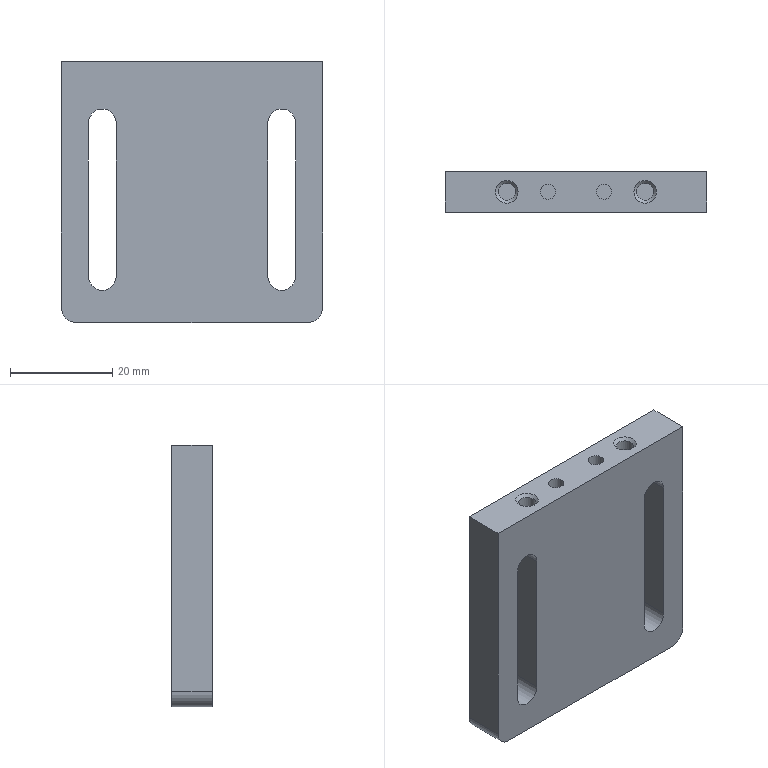Part | STEP file | ROTATION MC_NEW VER-0610_539 | 1 solid | 26 faces | box 51 x 8 x 51 mm | volume 17634 mm3 | plane 14 | cylinder 10 | cone 2 | commonest cylinder face diameters 5.4 x4 3 x2 3.3 x2 6 x2
STEP:
#1=CARTESIAN_POINT('',(200.831,612.268,-87.091));
#2=VERTEX_POINT('',#1);
#3=CARTESIAN_POINT('',(200.831,612.268,-57.091));
#4=VERTEX_POINT('',#3);
#5=CARTESIAN_POINT('',(200.831,612.268,-64.091));
#6=DIRECTION('',(0.,0.,1.));
#7=VECTOR('',#6,10.);
#8=LINE('',#5,#7);
#9=EDGE_CURVE('',#2,#4,#8,.T.);
#10=ORIENTED_EDGE('',*,*,#9,.F.);
#11=CARTESIAN_POINT('',(200.831,620.268,-87.091));
#12=VERTEX_POINT('',#11);
#13=CARTESIAN_POINT('',(200.831,620.268,-87.091));
#14=DIRECTION('',(0.,-1.,0.));
#15=VECTOR('',#14,10.);
#16=LINE('',#13,#15);
#17=EDGE_CURVE('',#12,#2,#16,.T.);
#18=ORIENTED_EDGE('',*,*,#17,.F.);
#19=CARTESIAN_POINT('',(200.831,620.268,-57.091));
#20=VERTEX_POINT('',#19);
#21=CARTESIAN_POINT('',(200.831,620.268,-64.091));
#22=DIRECTION('',(0.,0.,-1.));
#23=VECTOR('',#22,10.);
#24=LINE('',#21,#23);
#25=EDGE_CURVE('',#20,#12,#24,.T.);
#26=ORIENTED_EDGE('',*,*,#25,.F.);
#27=CARTESIAN_POINT('',(200.831,620.268,-57.091));
#28=DIRECTION('',(0.,-1.,0.));
#29=VECTOR('',#28,10.);
#30=LINE('',#27,#29);
#31=EDGE_CURVE('',#20,#4,#30,.T.);
#32=ORIENTED_EDGE('',*,*,#31,.T.);
#33=EDGE_LOOP('',(#10,#18,#26,#32));
#34=FACE_OUTER_BOUND('',#33,.T.);
#35=CARTESIAN_POINT('',(200.831,620.268,-87.091));
#36=DIRECTION('',(1.,0.,0.));
#37=DIRECTION('',(0.,0.,1.));
#38=AXIS2_PLACEMENT_3D('',#35,#36,#37);
#39=PLANE('',#38);
#40=ADVANCED_FACE('',(#34),#39,.T.);
#41=CARTESIAN_POINT('',(206.231,612.268,-87.091));
#42=VERTEX_POINT('',#41);
#43=CARTESIAN_POINT('',(203.531,612.268,-87.091));
#44=DIRECTION('',(0.,1.,0.));
#45=DIRECTION('',(-1.,0.,0.));
#46=AXIS2_PLACEMENT_3D('',#43,#44,#45);
#47=CIRCLE('',#46,2.7);
#48=EDGE_CURVE('',#42,#2,#47,.T.);
#49=ORIENTED_EDGE('',*,*,#48,.F.);
#50=CARTESIAN_POINT('',(206.231,620.268,-87.091));
#51=VERTEX_POINT('',#50);
#52=CARTESIAN_POINT('',(206.231,620.268,-87.091));
#53=DIRECTION('',(0.,-1.,0.));
#54=VECTOR('',#53,10.);
#55=LINE('',#52,#54);
#56=EDGE_CURVE('',#51,#42,#55,.T.);
#57=ORIENTED_EDGE('',*,*,#56,.F.);
#58=CARTESIAN_POINT('',(203.531,620.268,-87.091));
#59=DIRECTION('',(0.,-1.,0.));
#60=DIRECTION('',(-1.,0.,0.));
#61=AXIS2_PLACEMENT_3D('',#58,#59,#60);
#62=CIRCLE('',#61,2.7);
#63=EDGE_CURVE('',#12,#51,#62,.T.);
#64=ORIENTED_EDGE('',*,*,#63,.F.);
#65=ORIENTED_EDGE('',*,*,#17,.T.);
#66=EDGE_LOOP('',(#49,#57,#64,#65));
#67=FACE_OUTER_BOUND('',#66,.T.);
#68=CARTESIAN_POINT('',(203.531,620.268,-87.091));
#69=DIRECTION('',(0.,1.,0.));
#70=DIRECTION('',(-1.,0.,0.));
#71=AXIS2_PLACEMENT_3D('',#68,#69,#70);
#72=CYLINDRICAL_SURFACE('',#71,2.7);
#73=ADVANCED_FACE('',(#67),#72,.F.);
#74=CARTESIAN_POINT('',(206.231,612.268,-57.091));
#75=VERTEX_POINT('',#74);
#76=CARTESIAN_POINT('',(206.231,612.268,-49.091));
#77=DIRECTION('',(0.,0.,-1.));
#78=VECTOR('',#77,10.);
#79=LINE('',#76,#78);
#80=EDGE_CURVE('',#75,#42,#79,.T.);
#81=ORIENTED_EDGE('',*,*,#80,.F.);
#82=CARTESIAN_POINT('',(206.231,620.268,-57.091));
#83=VERTEX_POINT('',#82);
#84=CARTESIAN_POINT('',(206.231,620.268,-57.091));
#85=DIRECTION('',(0.,-1.,0.));
#86=VECTOR('',#85,10.);
#87=LINE('',#84,#86);
#88=EDGE_CURVE('',#83,#75,#87,.T.);
#89=ORIENTED_EDGE('',*,*,#88,.F.);
#90=CARTESIAN_POINT('',(206.231,620.268,-49.091));
#91=DIRECTION('',(0.,0.,1.));
#92=VECTOR('',#91,10.);
#93=LINE('',#90,#92);
#94=EDGE_CURVE('',#51,#83,#93,.T.);
#95=ORIENTED_EDGE('',*,*,#94,.F.);
#96=ORIENTED_EDGE('',*,*,#56,.T.);
#97=EDGE_LOOP('',(#81,#89,#95,#96));
#98=FACE_OUTER_BOUND('',#97,.T.);
#99=CARTESIAN_POINT('',(206.231,620.268,-57.091));
#100=DIRECTION('',(-1.,0.,0.));
#101=DIRECTION('',(0.,0.,-1.));
#102=AXIS2_PLACEMENT_3D('',#99,#100,#101);
#103=PLANE('',#102);
#104=ADVANCED_FACE('',(#98),#103,.T.);
#105=CARTESIAN_POINT('',(203.531,612.268,-57.091));
#106=DIRECTION('',(0.,1.,0.));
#107=DIRECTION('',(1.,0.,0.));
#108=AXIS2_PLACEMENT_3D('',#105,#106,#107);
#109=CIRCLE('',#108,2.7);
#110=EDGE_CURVE('',#4,#75,#109,.T.);
#111=ORIENTED_EDGE('',*,*,#110,.F.);
#112=ORIENTED_EDGE('',*,*,#31,.F.);
#113=CARTESIAN_POINT('',(203.531,620.268,-57.091));
#114=DIRECTION('',(0.,-1.,0.));
#115=DIRECTION('',(1.,0.,0.));
#116=AXIS2_PLACEMENT_3D('',#113,#114,#115);
#117=CIRCLE('',#116,2.7);
#118=EDGE_CURVE('',#83,#20,#117,.T.);
#119=ORIENTED_EDGE('',*,*,#118,.F.);
#120=ORIENTED_EDGE('',*,*,#88,.T.);
#121=EDGE_LOOP('',(#111,#112,#119,#120));
#122=FACE_OUTER_BOUND('',#121,.T.);
#123=CARTESIAN_POINT('',(203.531,620.268,-57.091));
#124=DIRECTION('',(0.,1.,0.));
#125=DIRECTION('',(1.,0.,0.));
#126=AXIS2_PLACEMENT_3D('',#123,#124,#125);
#127=CYLINDRICAL_SURFACE('',#126,2.7);
#128=ADVANCED_FACE('',(#122),#127,.F.);
#129=CARTESIAN_POINT('',(241.231,612.268,-57.091));
#130=VERTEX_POINT('',#129);
#131=CARTESIAN_POINT('',(241.231,612.268,-87.091));
#132=VERTEX_POINT('',#131);
#133=CARTESIAN_POINT('',(241.231,612.268,-64.091));
#134=DIRECTION('',(0.,0.,-1.));
#135=VECTOR('',#134,10.);
#136=LINE('',#133,#135);
#137=EDGE_CURVE('',#130,#132,#136,.T.);
#138=ORIENTED_EDGE('',*,*,#137,.F.);
#139=CARTESIAN_POINT('',(241.231,620.268,-57.091));
#140=VERTEX_POINT('',#139);
#141=CARTESIAN_POINT('',(241.231,620.268,-57.091));
#142=DIRECTION('',(0.,-1.,0.));
#143=VECTOR('',#142,10.);
#144=LINE('',#141,#143);
#145=EDGE_CURVE('',#140,#130,#144,.T.);
#146=ORIENTED_EDGE('',*,*,#145,.F.);
#147=CARTESIAN_POINT('',(241.231,620.268,-87.091));
#148=VERTEX_POINT('',#147);
#149=CARTESIAN_POINT('',(241.231,620.268,-64.091));
#150=DIRECTION('',(0.,0.,1.));
#151=VECTOR('',#150,10.);
#152=LINE('',#149,#151);
#153=EDGE_CURVE('',#148,#140,#152,.T.);
#154=ORIENTED_EDGE('',*,*,#153,.F.);
#155=CARTESIAN_POINT('',(241.231,620.268,-87.091));
#156=DIRECTION('',(0.,-1.,0.));
#157=VECTOR('',#156,10.);
#158=LINE('',#155,#157);
#159=EDGE_CURVE('',#148,#132,#158,.T.);
#160=ORIENTED_EDGE('',*,*,#159,.T.);
#161=EDGE_LOOP('',(#138,#146,#154,#160));
#162=FACE_OUTER_BOUND('',#161,.T.);
#163=CARTESIAN_POINT('',(241.231,620.268,-87.091));
#164=DIRECTION('',(1.,0.,0.));
#165=DIRECTION('',(0.,0.,1.));
#166=AXIS2_PLACEMENT_3D('',#163,#164,#165);
#167=PLANE('',#166);
#168=ADVANCED_FACE('',(#162),#167,.F.);
#169=CARTESIAN_POINT('',(235.831,612.268,-87.091));
#170=VERTEX_POINT('',#169);
#171=CARTESIAN_POINT('',(238.531,612.268,-87.091));
#172=DIRECTION('',(0.,1.,0.));
#173=DIRECTION('',(1.,0.,0.));
#174=AXIS2_PLACEMENT_3D('',#171,#172,#173);
#175=CIRCLE('',#174,2.7);
#176=EDGE_CURVE('',#132,#170,#175,.T.);
#177=ORIENTED_EDGE('',*,*,#176,.F.);
#178=ORIENTED_EDGE('',*,*,#159,.F.);
#179=CARTESIAN_POINT('',(235.831,620.268,-87.091));
#180=VERTEX_POINT('',#179);
#181=CARTESIAN_POINT('',(238.531,620.268,-87.091));
#182=DIRECTION('',(0.,-1.,0.));
#183=DIRECTION('',(1.,0.,0.));
#184=AXIS2_PLACEMENT_3D('',#181,#182,#183);
#185=CIRCLE('',#184,2.7);
#186=EDGE_CURVE('',#180,#148,#185,.T.);
#187=ORIENTED_EDGE('',*,*,#186,.F.);
#188=CARTESIAN_POINT('',(235.831,620.268,-87.091));
#189=DIRECTION('',(0.,-1.,0.));
#190=VECTOR('',#189,10.);
#191=LINE('',#188,#190);
#192=EDGE_CURVE('',#180,#170,#191,.T.);
#193=ORIENTED_EDGE('',*,*,#192,.T.);
#194=EDGE_LOOP('',(#177,#178,#187,#193));
#195=FACE_OUTER_BOUND('',#194,.T.);
#196=CARTESIAN_POINT('',(238.531,620.268,-87.091));
#197=DIRECTION('',(0.,-1.,0.));
#198=DIRECTION('',(1.,0.,0.));
#199=AXIS2_PLACEMENT_3D('',#196,#197,#198);
#200=CYLINDRICAL_SURFACE('',#199,2.7);
#201=ADVANCED_FACE('',(#195),#200,.F.);
#202=CARTESIAN_POINT('',(235.831,612.268,-57.091));
#203=VERTEX_POINT('',#202);
#204=CARTESIAN_POINT('',(235.831,612.268,-49.091));
#205=DIRECTION('',(0.,0.,1.));
#206=VECTOR('',#205,10.);
#207=LINE('',#204,#206);
#208=EDGE_CURVE('',#170,#203,#207,.T.);
#209=ORIENTED_EDGE('',*,*,#208,.F.);
#210=ORIENTED_EDGE('',*,*,#192,.F.);
#211=CARTESIAN_POINT('',(235.831,620.268,-57.091));
#212=VERTEX_POINT('',#211);
#213=CARTESIAN_POINT('',(235.831,620.268,-49.091));
#214=DIRECTION('',(0.,0.,-1.));
#215=VECTOR('',#214,10.);
#216=LINE('',#213,#215);
#217=EDGE_CURVE('',#212,#180,#216,.T.);
#218=ORIENTED_EDGE('',*,*,#217,.F.);
#219=CARTESIAN_POINT('',(235.831,620.268,-57.091));
#220=DIRECTION('',(0.,-1.,0.));
#221=VECTOR('',#220,10.);
#222=LINE('',#219,#221);
#223=EDGE_CURVE('',#212,#203,#222,.T.);
#224=ORIENTED_EDGE('',*,*,#223,.T.);
#225=EDGE_LOOP('',(#209,#210,#218,#224));
#226=FACE_OUTER_BOUND('',#225,.T.);
#227=CARTESIAN_POINT('',(235.831,620.268,-57.091));
#228=DIRECTION('',(-1.,0.,0.));
#229=DIRECTION('',(0.,0.,-1.));
#230=AXIS2_PLACEMENT_3D('',#227,#228,#229);
#231=PLANE('',#230);
#232=ADVANCED_FACE('',(#226),#231,.F.);
#233=CARTESIAN_POINT('',(238.531,612.268,-57.091));
#234=DIRECTION('',(0.,1.,0.));
#235=DIRECTION('',(-1.,0.,0.));
#236=AXIS2_PLACEMENT_3D('',#233,#234,#235);
#237=CIRCLE('',#236,2.7);
#238=EDGE_CURVE('',#203,#130,#237,.T.);
#239=ORIENTED_EDGE('',*,*,#238,.F.);
#240=ORIENTED_EDGE('',*,*,#223,.F.);
#241=CARTESIAN_POINT('',(238.531,620.268,-57.091));
#242=DIRECTION('',(0.,-1.,0.));
#243=DIRECTION('',(-1.,0.,0.));
#244=AXIS2_PLACEMENT_3D('',#241,#242,#243);
#245=CIRCLE('',#244,2.7);
#246=EDGE_CURVE('',#140,#212,#245,.T.);
#247=ORIENTED_EDGE('',*,*,#246,.F.);
#248=ORIENTED_EDGE('',*,*,#145,.T.);
#249=EDGE_LOOP('',(#239,#240,#247,#248));
#250=FACE_OUTER_BOUND('',#249,.T.);
#251=CARTESIAN_POINT('',(238.531,620.268,-57.091));
#252=DIRECTION('',(0.,-1.,0.));
#253=DIRECTION('',(-1.,0.,0.));
#254=AXIS2_PLACEMENT_3D('',#251,#252,#253);
#255=CYLINDRICAL_SURFACE('',#254,2.7);
#256=ADVANCED_FACE('',(#250),#255,.F.);
#257=CARTESIAN_POINT('',(195.531,620.268,-93.091));
#258=VERTEX_POINT('',#257);
#259=CARTESIAN_POINT('',(198.531,620.268,-96.091));
#260=VERTEX_POINT('',#259);
#261=CARTESIAN_POINT('',(198.531,620.268,-93.091));
#262=DIRECTION('',(0.,-1.,0.));
#263=DIRECTION('',(-0.7071,0.,-0.7071));
#264=AXIS2_PLACEMENT_3D('',#261,#262,#263);
#265=CIRCLE('',#264,3.);
#266=EDGE_CURVE('',#258,#260,#265,.T.);
#267=ORIENTED_EDGE('',*,*,#266,.T.);
#268=CARTESIAN_POINT('',(198.531,612.268,-96.091));
#269=VERTEX_POINT('',#268);
#270=CARTESIAN_POINT('',(198.531,612.268,-96.091));
#271=DIRECTION('',(0.,-1.,0.));
#272=VECTOR('',#271,10.);
#273=LINE('',#270,#272);
#274=EDGE_CURVE('',#260,#269,#273,.T.);
#275=ORIENTED_EDGE('',*,*,#274,.T.);
#276=CARTESIAN_POINT('',(195.531,612.268,-93.091));
#277=VERTEX_POINT('',#276);
#278=CARTESIAN_POINT('',(198.531,612.268,-93.091));
#279=DIRECTION('',(0.,1.,0.));
#280=DIRECTION('',(-0.7071,0.,-0.7071));
#281=AXIS2_PLACEMENT_3D('',#278,#279,#280);
#282=CIRCLE('',#281,3.);
#283=EDGE_CURVE('',#269,#277,#282,.T.);
#284=ORIENTED_EDGE('',*,*,#283,.T.);
#285=CARTESIAN_POINT('',(195.531,612.268,-93.091));
#286=DIRECTION('',(0.,1.,0.));
#287=VECTOR('',#286,10.);
#288=LINE('',#285,#287);
#289=EDGE_CURVE('',#277,#258,#288,.T.);
#290=ORIENTED_EDGE('',*,*,#289,.T.);
#291=EDGE_LOOP('',(#267,#275,#284,#290));
#292=FACE_OUTER_BOUND('',#291,.T.);
#293=CARTESIAN_POINT('',(198.531,612.268,-93.091));
#294=DIRECTION('',(0.,1.,0.));
#295=DIRECTION('',(-0.7071,0.,-0.7071));
#296=AXIS2_PLACEMENT_3D('',#293,#294,#295);
#297=CYLINDRICAL_SURFACE('',#296,3.);
#298=ADVANCED_FACE('',(#292),#297,.T.);
#299=ORIENTED_EDGE('',*,*,#289,.F.);
#300=CARTESIAN_POINT('',(195.531,612.268,-45.091));
#301=VERTEX_POINT('',#300);
#302=CARTESIAN_POINT('',(195.531,612.268,-45.091));
#303=DIRECTION('',(0.,0.,-1.));
#304=VECTOR('',#303,33.);
#305=LINE('',#302,#304);
#306=EDGE_CURVE('',#301,#277,#305,.T.);
#307=ORIENTED_EDGE('',*,*,#306,.F.);
#308=CARTESIAN_POINT('',(195.531,620.268,-45.091));
#309=VERTEX_POINT('',#308);
#310=CARTESIAN_POINT('',(195.531,612.268,-45.091));
#311=DIRECTION('',(0.,1.,0.));
#312=VECTOR('',#311,8.);
#313=LINE('',#310,#312);
#314=EDGE_CURVE('',#301,#309,#313,.T.);
#315=ORIENTED_EDGE('',*,*,#314,.T.);
#316=CARTESIAN_POINT('',(195.531,620.268,-45.091));
#317=DIRECTION('',(0.,0.,-1.));
#318=VECTOR('',#317,33.);
#319=LINE('',#316,#318);
#320=EDGE_CURVE('',#309,#258,#319,.T.);
#321=ORIENTED_EDGE('',*,*,#320,.T.);
#322=EDGE_LOOP('',(#299,#307,#315,#321));
#323=FACE_OUTER_BOUND('',#322,.T.);
#324=CARTESIAN_POINT('',(195.531,612.268,-67.091));
#325=DIRECTION('',(-1.,0.,0.));
#326=DIRECTION('',(0.,0.,1.));
#327=AXIS2_PLACEMENT_3D('',#324,#325,#326);
#328=PLANE('',#327);
#329=ADVANCED_FACE('',(#323),#328,.T.);
#330=ORIENTED_EDGE('',*,*,#283,.F.);
#331=CARTESIAN_POINT('',(243.531,612.268,-96.091));
#332=VERTEX_POINT('',#331);
#333=CARTESIAN_POINT('',(198.531,612.268,-96.091));
#334=DIRECTION('',(1.,0.,0.));
#335=VECTOR('',#334,45.);
#336=LINE('',#333,#335);
#337=EDGE_CURVE('',#269,#332,#336,.T.);
#338=ORIENTED_EDGE('',*,*,#337,.T.);
#339=CARTESIAN_POINT('',(246.531,612.268,-93.091));
#340=VERTEX_POINT('',#339);
#341=CARTESIAN_POINT('',(243.531,612.268,-93.091));
#342=DIRECTION('',(0.,1.,0.));
#343=DIRECTION('',(0.7071,0.,-0.7071));
#344=AXIS2_PLACEMENT_3D('',#341,#342,#343);
#345=CIRCLE('',#344,3.);
#346=EDGE_CURVE('',#340,#332,#345,.T.);
#347=ORIENTED_EDGE('',*,*,#346,.F.);
#348=CARTESIAN_POINT('',(246.531,612.268,-45.091));
#349=VERTEX_POINT('',#348);
#350=CARTESIAN_POINT('',(246.531,612.268,-45.091));
#351=DIRECTION('',(0.,0.,-1.));
#352=VECTOR('',#351,33.);
#353=LINE('',#350,#352);
#354=EDGE_CURVE('',#349,#340,#353,.T.);
#355=ORIENTED_EDGE('',*,*,#354,.F.);
#356=CARTESIAN_POINT('',(246.531,612.268,-45.091));
#357=DIRECTION('',(-1.,0.,0.));
#358=VECTOR('',#357,51.);
#359=LINE('',#356,#358);
#360=EDGE_CURVE('',#349,#301,#359,.T.);
#361=ORIENTED_EDGE('',*,*,#360,.T.);
#362=ORIENTED_EDGE('',*,*,#306,.T.);
#363=EDGE_LOOP('',(#330,#338,#347,#355,#361,#362));
#364=FACE_OUTER_BOUND('',#363,.T.);
#365=ORIENTED_EDGE('',*,*,#9,.T.);
#366=ORIENTED_EDGE('',*,*,#110,.T.);
#367=ORIENTED_EDGE('',*,*,#80,.T.);
#368=ORIENTED_EDGE('',*,*,#48,.T.);
#369=EDGE_LOOP('',(#365,#366,#367,#368));
#370=FACE_BOUND('',#369,.T.);
#371=ORIENTED_EDGE('',*,*,#208,.T.);
#372=ORIENTED_EDGE('',*,*,#238,.T.);
#373=ORIENTED_EDGE('',*,*,#137,.T.);
#374=ORIENTED_EDGE('',*,*,#176,.T.);
#375=EDGE_LOOP('',(#371,#372,#373,#374));
#376=FACE_BOUND('',#375,.T.);
#377=CARTESIAN_POINT('',(208.417,612.268,-41.091));
#378=DIRECTION('',(0.,1.,0.));
#379=DIRECTION('',(0.,0.,1.));
#380=AXIS2_PLACEMENT_3D('',#377,#378,#379);
#381=PLANE('',#380);
#382=ADVANCED_FACE('',(#364,#370,#376),#381,.F.);
#383=CARTESIAN_POINT('',(243.531,620.268,-96.091));
#384=VERTEX_POINT('',#383);
#385=CARTESIAN_POINT('',(246.531,620.268,-93.091));
#386=VERTEX_POINT('',#385);
#387=CARTESIAN_POINT('',(243.531,620.268,-93.091));
#388=DIRECTION('',(0.,-1.,0.));
#389=DIRECTION('',(0.7071,0.,-0.7071));
#390=AXIS2_PLACEMENT_3D('',#387,#388,#389);
#391=CIRCLE('',#390,3.);
#392=EDGE_CURVE('',#384,#386,#391,.T.);
#393=ORIENTED_EDGE('',*,*,#392,.T.);
#394=CARTESIAN_POINT('',(246.531,612.268,-93.091));
#395=DIRECTION('',(0.,-1.,0.));
#396=VECTOR('',#395,10.);
#397=LINE('',#394,#396);
#398=EDGE_CURVE('',#386,#340,#397,.T.);
#399=ORIENTED_EDGE('',*,*,#398,.T.);
#400=ORIENTED_EDGE('',*,*,#346,.T.);
#401=CARTESIAN_POINT('',(243.531,612.268,-96.091));
#402=DIRECTION('',(0.,1.,0.));
#403=VECTOR('',#402,10.);
#404=LINE('',#401,#403);
#405=EDGE_CURVE('',#332,#384,#404,.T.);
#406=ORIENTED_EDGE('',*,*,#405,.T.);
#407=EDGE_LOOP('',(#393,#399,#400,#406));
#408=FACE_OUTER_BOUND('',#407,.T.);
#409=CARTESIAN_POINT('',(243.531,612.268,-93.091));
#410=DIRECTION('',(0.,1.,0.));
#411=DIRECTION('',(0.7071,0.,-0.7071));
#412=AXIS2_PLACEMENT_3D('',#409,#410,#411);
#413=CYLINDRICAL_SURFACE('',#412,3.);
#414=ADVANCED_FACE('',(#408),#413,.T.);
#415=ORIENTED_EDGE('',*,*,#398,.F.);
#416=CARTESIAN_POINT('',(246.531,620.268,-45.091));
#417=VERTEX_POINT('',#416);
#418=CARTESIAN_POINT('',(246.531,620.268,-45.091));
#419=DIRECTION('',(0.,0.,-1.));
#420=VECTOR('',#419,33.);
#421=LINE('',#418,#420);
#422=EDGE_CURVE('',#417,#386,#421,.T.);
#423=ORIENTED_EDGE('',*,*,#422,.F.);
#424=CARTESIAN_POINT('',(246.531,620.268,-45.091));
#425=DIRECTION('',(0.,-1.,0.));
#426=VECTOR('',#425,8.);
#427=LINE('',#424,#426);
#428=EDGE_CURVE('',#417,#349,#427,.T.);
#429=ORIENTED_EDGE('',*,*,#428,.T.);
#430=ORIENTED_EDGE('',*,*,#354,.T.);
#431=EDGE_LOOP('',(#415,#423,#429,#430));
#432=FACE_OUTER_BOUND('',#431,.T.);
#433=CARTESIAN_POINT('',(246.531,612.268,-67.091));
#434=DIRECTION('',(1.,0.,0.));
#435=DIRECTION('',(0.,0.,-1.));
#436=AXIS2_PLACEMENT_3D('',#433,#434,#435);
#437=PLANE('',#436);
#438=ADVANCED_FACE('',(#432),#437,.T.);
#439=ORIENTED_EDGE('',*,*,#274,.F.);
#440=CARTESIAN_POINT('',(243.531,620.268,-96.091));
#441=DIRECTION('',(-1.,0.,0.));
#442=VECTOR('',#441,45.);
#443=LINE('',#440,#442);
#444=EDGE_CURVE('',#384,#260,#443,.T.);
#445=ORIENTED_EDGE('',*,*,#444,.F.);
#446=ORIENTED_EDGE('',*,*,#405,.F.);
#447=ORIENTED_EDGE('',*,*,#337,.F.);
#448=EDGE_LOOP('',(#439,#445,#446,#447));
#449=FACE_OUTER_BOUND('',#448,.T.);
#450=CARTESIAN_POINT('',(223.917,612.268,-96.091));
#451=DIRECTION('',(0.,0.,-1.));
#452=DIRECTION('',(-1.,0.,0.));
#453=AXIS2_PLACEMENT_3D('',#450,#451,#452);
#454=PLANE('',#453);
#455=ADVANCED_FACE('',(#449),#454,.T.);
#456=CARTESIAN_POINT('',(217.031,616.268,-50.351));
#457=VERTEX_POINT('',#456);
#458=CARTESIAN_POINT('',(215.531,616.268,-50.351));
#459=DIRECTION('',(0.,0.,-1.));
#460=DIRECTION('',(1.,0.,0.));
#461=AXIS2_PLACEMENT_3D('',#458,#459,#460);
#462=CIRCLE('',#461,1.5);
#463=EDGE_CURVE('',#457,#457,#462,.T.);
#464=ORIENTED_EDGE('',*,*,#463,.F.);
#465=EDGE_LOOP('',(#464));
#466=FACE_OUTER_BOUND('',#465,.T.);
#467=CARTESIAN_POINT('',(235.031,620.268,-50.351));
#468=DIRECTION('',(0.,0.,-1.));
#469=DIRECTION('',(-1.,0.,0.));
#470=AXIS2_PLACEMENT_3D('',#467,#468,#469);
#471=PLANE('',#470);
#472=ADVANCED_FACE('',(#466),#471,.F.);
#473=CARTESIAN_POINT('',(228.031,616.268,-50.351));
#474=VERTEX_POINT('',#473);
#475=CARTESIAN_POINT('',(226.531,616.268,-50.351));
#476=DIRECTION('',(0.,0.,-1.));
#477=DIRECTION('',(1.,0.,0.));
#478=AXIS2_PLACEMENT_3D('',#475,#476,#477);
#479=CIRCLE('',#478,1.5);
#480=EDGE_CURVE('',#474,#474,#479,.T.);
#481=ORIENTED_EDGE('',*,*,#480,.T.);
#482=CARTESIAN_POINT('',(228.031,616.268,-45.091));
#483=VERTEX_POINT('',#482);
#484=CARTESIAN_POINT('',(228.031,616.268,-24.091));
#485=DIRECTION('',(0.,0.,1.));
#486=VECTOR('',#485,1.5);
#487=LINE('',#484,#486);
#488=EDGE_CURVE('',#474,#483,#487,.T.);
#489=ORIENTED_EDGE('',*,*,#488,.T.);
#490=CARTESIAN_POINT('',(226.531,616.268,-45.091));
#491=DIRECTION('',(0.,0.,1.));
#492=DIRECTION('',(1.,0.,0.));
#493=AXIS2_PLACEMENT_3D('',#490,#491,#492);
#494=CIRCLE('',#493,1.5);
#495=EDGE_CURVE('',#483,#483,#494,.T.);
#496=ORIENTED_EDGE('',*,*,#495,.T.);
#497=ORIENTED_EDGE('',*,*,#488,.F.);
#498=EDGE_LOOP('',(#481,#489,#496,#497));
#499=FACE_OUTER_BOUND('',#498,.T.);
#500=CARTESIAN_POINT('',(226.531,616.268,-24.091));
#501=DIRECTION('',(0.,0.,1.));
#502=DIRECTION('',(-1.,0.,0.));
#503=AXIS2_PLACEMENT_3D('',#500,#501,#502);
#504=CYLINDRICAL_SURFACE('',#503,1.5);
#505=ADVANCED_FACE('',(#499),#504,.F.);
#506=ORIENTED_EDGE('',*,*,#266,.F.);
#507=ORIENTED_EDGE('',*,*,#320,.F.);
#508=CARTESIAN_POINT('',(195.531,620.268,-45.091));
#509=DIRECTION('',(1.,0.,0.));
#510=VECTOR('',#509,51.);
#511=LINE('',#508,#510);
#512=EDGE_CURVE('',#309,#417,#511,.T.);
#513=ORIENTED_EDGE('',*,*,#512,.T.);
#514=ORIENTED_EDGE('',*,*,#422,.T.);
#515=ORIENTED_EDGE('',*,*,#392,.F.);
#516=ORIENTED_EDGE('',*,*,#444,.T.);
#517=EDGE_LOOP('',(#506,#507,#513,#514,#515,#516));
#518=FACE_OUTER_BOUND('',#517,.T.);
#519=ORIENTED_EDGE('',*,*,#25,.T.);
#520=ORIENTED_EDGE('',*,*,#63,.T.);
#521=ORIENTED_EDGE('',*,*,#94,.T.);
#522=ORIENTED_EDGE('',*,*,#118,.T.);
#523=EDGE_LOOP('',(#519,#520,#521,#522));
#524=FACE_BOUND('',#523,.T.);
#525=ORIENTED_EDGE('',*,*,#217,.T.);
#526=ORIENTED_EDGE('',*,*,#186,.T.);
#527=ORIENTED_EDGE('',*,*,#153,.T.);
#528=ORIENTED_EDGE('',*,*,#246,.T.);
#529=EDGE_LOOP('',(#525,#526,#527,#528));
#530=FACE_BOUND('',#529,.T.);
#531=CARTESIAN_POINT('',(208.417,620.268,-41.091));
#532=DIRECTION('',(0.,1.,0.));
#533=DIRECTION('',(0.,0.,1.));
#534=AXIS2_PLACEMENT_3D('',#531,#532,#533);
#535=PLANE('',#534);
#536=ADVANCED_FACE('',(#518,#524,#530),#535,.T.);
#537=ORIENTED_EDGE('',*,*,#463,.T.);
#538=CARTESIAN_POINT('',(217.031,616.268,-45.091));
#539=VERTEX_POINT('',#538);
#540=CARTESIAN_POINT('',(217.031,616.268,-24.091));
#541=DIRECTION('',(0.,0.,1.));
#542=VECTOR('',#541,1.5);
#543=LINE('',#540,#542);
#544=EDGE_CURVE('',#457,#539,#543,.T.);
#545=ORIENTED_EDGE('',*,*,#544,.T.);
#546=CARTESIAN_POINT('',(215.531,616.268,-45.091));
#547=DIRECTION('',(0.,0.,1.));
#548=DIRECTION('',(1.,0.,0.));
#549=AXIS2_PLACEMENT_3D('',#546,#547,#548);
#550=CIRCLE('',#549,1.5);
#551=EDGE_CURVE('',#539,#539,#550,.T.);
#552=ORIENTED_EDGE('',*,*,#551,.T.);
#553=ORIENTED_EDGE('',*,*,#544,.F.);
#554=EDGE_LOOP('',(#537,#545,#552,#553));
#555=FACE_OUTER_BOUND('',#554,.T.);
#556=CARTESIAN_POINT('',(215.531,616.268,-24.091));
#557=DIRECTION('',(0.,0.,1.));
#558=DIRECTION('',(-1.,0.,0.));
#559=AXIS2_PLACEMENT_3D('',#556,#557,#558);
#560=CYLINDRICAL_SURFACE('',#559,1.5);
#561=ADVANCED_FACE('',(#555),#560,.F.);
#562=CARTESIAN_POINT('',(209.181,616.268,-45.651));
#563=VERTEX_POINT('',#562);
#564=CARTESIAN_POINT('',(205.881,616.268,-45.651));
#565=VERTEX_POINT('',#564);
#566=CARTESIAN_POINT('',(207.531,616.268,-45.651));
#567=DIRECTION('',(0.,0.,-1.));
#568=DIRECTION('',(-1.,0.,0.));
#569=AXIS2_PLACEMENT_3D('',#566,#567,#568);
#570=CIRCLE('',#569,1.65);
#571=EDGE_CURVE('',#563,#565,#570,.T.);
#572=ORIENTED_EDGE('',*,*,#571,.T.);
#573=CARTESIAN_POINT('',(205.321,616.268,-45.091));
#574=VERTEX_POINT('',#573);
#575=CARTESIAN_POINT('',(205.581,616.268,-45.351));
#576=DIRECTION('',(-0.7071,0.,0.7071));
#577=VECTOR('',#576,1.95);
#578=LINE('',#575,#577);
#579=EDGE_CURVE('',#565,#574,#578,.T.);
#580=ORIENTED_EDGE('',*,*,#579,.T.);
#581=CARTESIAN_POINT('',(207.531,616.268,-45.091));
#582=DIRECTION('',(0.,0.,1.));
#583=DIRECTION('',(0.,1.,0.));
#584=AXIS2_PLACEMENT_3D('',#581,#582,#583);
#585=CIRCLE('',#584,2.21);
#586=EDGE_CURVE('',#574,#574,#585,.T.);
#587=ORIENTED_EDGE('',*,*,#586,.T.);
#588=ORIENTED_EDGE('',*,*,#579,.F.);
#589=CARTESIAN_POINT('',(207.531,616.268,-45.651));
#590=DIRECTION('',(0.,0.,-1.));
#591=DIRECTION('',(-1.,0.,0.));
#592=AXIS2_PLACEMENT_3D('',#589,#590,#591);
#593=CIRCLE('',#592,1.65);
#594=EDGE_CURVE('',#565,#563,#593,.T.);
#595=ORIENTED_EDGE('',*,*,#594,.T.);
#596=EDGE_LOOP('',(#572,#580,#587,#588,#595));
#597=FACE_OUTER_BOUND('',#596,.T.);
#598=CARTESIAN_POINT('',(207.531,616.268,-45.351));
#599=DIRECTION('',(0.,0.,1.));
#600=DIRECTION('',(1.,0.,0.));
#601=AXIS2_PLACEMENT_3D('',#598,#599,#600);
#602=CONICAL_SURFACE('',#601,1.95,0.7854);
#603=ADVANCED_FACE('',(#597),#602,.F.);
#604=CARTESIAN_POINT('',(209.181,616.268,-51.351));
#605=VERTEX_POINT('',#604);
#606=CARTESIAN_POINT('',(207.531,616.268,-51.351));
#607=DIRECTION('',(0.,0.,-1.));
#608=DIRECTION('',(1.,0.,0.));
#609=AXIS2_PLACEMENT_3D('',#606,#607,#608);
#610=CIRCLE('',#609,1.65);
#611=EDGE_CURVE('',#605,#605,#610,.T.);
#612=ORIENTED_EDGE('',*,*,#611,.F.);
#613=EDGE_LOOP('',(#612));
#614=FACE_OUTER_BOUND('',#613,.T.);
#615=CARTESIAN_POINT('',(227.031,620.268,-51.351));
#616=DIRECTION('',(0.,0.,-1.));
#617=DIRECTION('',(-1.,0.,0.));
#618=AXIS2_PLACEMENT_3D('',#615,#616,#617);
#619=PLANE('',#618);
#620=ADVANCED_FACE('',(#614),#619,.F.);
#621=CARTESIAN_POINT('',(236.181,616.268,-51.351));
#622=VERTEX_POINT('',#621);
#623=CARTESIAN_POINT('',(234.531,616.268,-51.351));
#624=DIRECTION('',(0.,0.,-1.));
#625=DIRECTION('',(1.,0.,0.));
#626=AXIS2_PLACEMENT_3D('',#623,#624,#625);
#627=CIRCLE('',#626,1.65);
#628=EDGE_CURVE('',#622,#622,#627,.T.);
#629=ORIENTED_EDGE('',*,*,#628,.F.);
#630=EDGE_LOOP('',(#629));
#631=FACE_OUTER_BOUND('',#630,.T.);
#632=CARTESIAN_POINT('',(254.031,620.268,-51.351));
#633=DIRECTION('',(0.,0.,-1.));
#634=DIRECTION('',(-1.,0.,0.));
#635=AXIS2_PLACEMENT_3D('',#632,#633,#634);
#636=PLANE('',#635);
#637=ADVANCED_FACE('',(#631),#636,.F.);
#638=ORIENTED_EDGE('',*,*,#628,.T.);
#639=CARTESIAN_POINT('',(236.181,616.268,-45.651));
#640=VERTEX_POINT('',#639);
#641=CARTESIAN_POINT('',(236.181,616.268,-24.091));
#642=DIRECTION('',(0.,0.,1.));
#643=VECTOR('',#642,1.65);
#644=LINE('',#641,#643);
#645=EDGE_CURVE('',#622,#640,#644,.T.);
#646=ORIENTED_EDGE('',*,*,#645,.T.);
#647=CARTESIAN_POINT('',(232.881,616.268,-45.651));
#648=VERTEX_POINT('',#647);
#649=CARTESIAN_POINT('',(234.531,616.268,-45.651));
#650=DIRECTION('',(0.,0.,-1.));
#651=DIRECTION('',(-1.,0.,0.));
#652=AXIS2_PLACEMENT_3D('',#649,#650,#651);
#653=CIRCLE('',#652,1.65);
#654=EDGE_CURVE('',#648,#640,#653,.T.);
#655=ORIENTED_EDGE('',*,*,#654,.F.);
#656=CARTESIAN_POINT('',(234.531,616.268,-45.651));
#657=DIRECTION('',(0.,0.,-1.));
#658=DIRECTION('',(-1.,0.,0.));
#659=AXIS2_PLACEMENT_3D('',#656,#657,#658);
#660=CIRCLE('',#659,1.65);
#661=EDGE_CURVE('',#640,#648,#660,.T.);
#662=ORIENTED_EDGE('',*,*,#661,.F.);
#663=ORIENTED_EDGE('',*,*,#645,.F.);
#664=EDGE_LOOP('',(#638,#646,#655,#662,#663));
#665=FACE_OUTER_BOUND('',#664,.T.);
#666=CARTESIAN_POINT('',(234.531,616.268,-24.091));
#667=DIRECTION('',(0.,0.,1.));
#668=DIRECTION('',(-1.,0.,0.));
#669=AXIS2_PLACEMENT_3D('',#666,#667,#668);
#670=CYLINDRICAL_SURFACE('',#669,1.65);
#671=ADVANCED_FACE('',(#665),#670,.F.);
#672=ORIENTED_EDGE('',*,*,#480,.F.);
#673=EDGE_LOOP('',(#672));
#674=FACE_OUTER_BOUND('',#673,.T.);
#675=CARTESIAN_POINT('',(246.031,620.268,-50.351));
#676=DIRECTION('',(0.,0.,-1.));
#677=DIRECTION('',(-1.,0.,0.));
#678=AXIS2_PLACEMENT_3D('',#675,#676,#677);
#679=PLANE('',#678);
#680=ADVANCED_FACE('',(#674),#679,.F.);
#681=ORIENTED_EDGE('',*,*,#611,.T.);
#682=CARTESIAN_POINT('',(209.181,616.268,-24.091));
#683=DIRECTION('',(0.,0.,1.));
#684=VECTOR('',#683,1.65);
#685=LINE('',#682,#684);
#686=EDGE_CURVE('',#605,#563,#685,.T.);
#687=ORIENTED_EDGE('',*,*,#686,.T.);
#688=ORIENTED_EDGE('',*,*,#594,.F.);
#689=ORIENTED_EDGE('',*,*,#571,.F.);
#690=ORIENTED_EDGE('',*,*,#686,.F.);
#691=EDGE_LOOP('',(#681,#687,#688,#689,#690));
#692=FACE_OUTER_BOUND('',#691,.T.);
#693=CARTESIAN_POINT('',(207.531,616.268,-24.091));
#694=DIRECTION('',(0.,0.,1.));
#695=DIRECTION('',(-1.,0.,0.));
#696=AXIS2_PLACEMENT_3D('',#693,#694,#695);
#697=CYLINDRICAL_SURFACE('',#696,1.65);
#698=ADVANCED_FACE('',(#692),#697,.F.);
#699=ORIENTED_EDGE('',*,*,#654,.T.);
#700=ORIENTED_EDGE('',*,*,#661,.T.);
#701=CARTESIAN_POINT('',(232.321,616.268,-45.091));
#702=VERTEX_POINT('',#701);
#703=CARTESIAN_POINT('',(232.581,616.268,-45.351));
#704=DIRECTION('',(-0.7071,0.,0.7071));
#705=VECTOR('',#704,1.95);
#706=LINE('',#703,#705);
#707=EDGE_CURVE('',#648,#702,#706,.T.);
#708=ORIENTED_EDGE('',*,*,#707,.T.);
#709=CARTESIAN_POINT('',(234.531,616.268,-45.091));
#710=DIRECTION('',(0.,0.,1.));
#711=DIRECTION('',(0.,1.,0.));
#712=AXIS2_PLACEMENT_3D('',#709,#710,#711);
#713=CIRCLE('',#712,2.21);
#714=EDGE_CURVE('',#702,#702,#713,.T.);
#715=ORIENTED_EDGE('',*,*,#714,.T.);
#716=ORIENTED_EDGE('',*,*,#707,.F.);
#717=EDGE_LOOP('',(#699,#700,#708,#715,#716));
#718=FACE_OUTER_BOUND('',#717,.T.);
#719=CARTESIAN_POINT('',(234.531,616.268,-45.351));
#720=DIRECTION('',(0.,0.,1.));
#721=DIRECTION('',(1.,0.,0.));
#722=AXIS2_PLACEMENT_3D('',#719,#720,#721);
#723=CONICAL_SURFACE('',#722,1.95,0.7854);
#724=ADVANCED_FACE('',(#718),#723,.F.);
#725=ORIENTED_EDGE('',*,*,#428,.F.);
#726=ORIENTED_EDGE('',*,*,#512,.F.);
#727=ORIENTED_EDGE('',*,*,#314,.F.);
#728=ORIENTED_EDGE('',*,*,#360,.F.);
#729=EDGE_LOOP('',(#725,#726,#727,#728));
#730=FACE_OUTER_BOUND('',#729,.T.);
#731=ORIENTED_EDGE('',*,*,#495,.F.);
#732=EDGE_LOOP('',(#731));
#733=FACE_BOUND('',#732,.T.);
#734=ORIENTED_EDGE('',*,*,#551,.F.);
#735=EDGE_LOOP('',(#734));
#736=FACE_BOUND('',#735,.T.);
#737=ORIENTED_EDGE('',*,*,#586,.F.);
#738=EDGE_LOOP('',(#737));
#739=FACE_BOUND('',#738,.T.);
#740=ORIENTED_EDGE('',*,*,#714,.F.);
#741=EDGE_LOOP('',(#740));
#742=FACE_BOUND('',#741,.T.);
#743=CARTESIAN_POINT('',(227.031,620.268,-45.091));
#744=DIRECTION('',(0.,0.,-1.));
#745=DIRECTION('',(-1.,0.,0.));
#746=AXIS2_PLACEMENT_3D('',#743,#744,#745);
#747=PLANE('',#746);
#748=ADVANCED_FACE('',(#730,#733,#736,#739,#742),#747,.F.);
#749=CLOSED_SHELL('',(#40,#73,#104,#128,#168,#201,#232,#256,#298,#329,#382,#414,#438,#455,#472,#505,#536,#561,#603,#620,#637,#671,#680,#698,#724,#748));
#750=MANIFOLD_SOLID_BREP('',#749);
#751=(LENGTH_UNIT()NAMED_UNIT(*)SI_UNIT(.MILLI.,.METRE.));
#752=UNCERTAINTY_MEASURE_WITH_UNIT(LENGTH_MEASURE(0.01),#751,'','');
#753=(NAMED_UNIT(*)PLANE_ANGLE_UNIT()SI_UNIT($,.RADIAN.));
#754=(NAMED_UNIT(*)SI_UNIT($,.STERADIAN.)SOLID_ANGLE_UNIT());
#755=(GEOMETRIC_REPRESENTATION_CONTEXT(3)GLOBAL_UNCERTAINTY_ASSIGNED_CONTEXT((#752))GLOBAL_UNIT_ASSIGNED_CONTEXT((#751,#753,#754))REPRESENTATION_CONTEXT('',''));
#756=ADVANCED_BREP_SHAPE_REPRESENTATION('',(#750),#755);